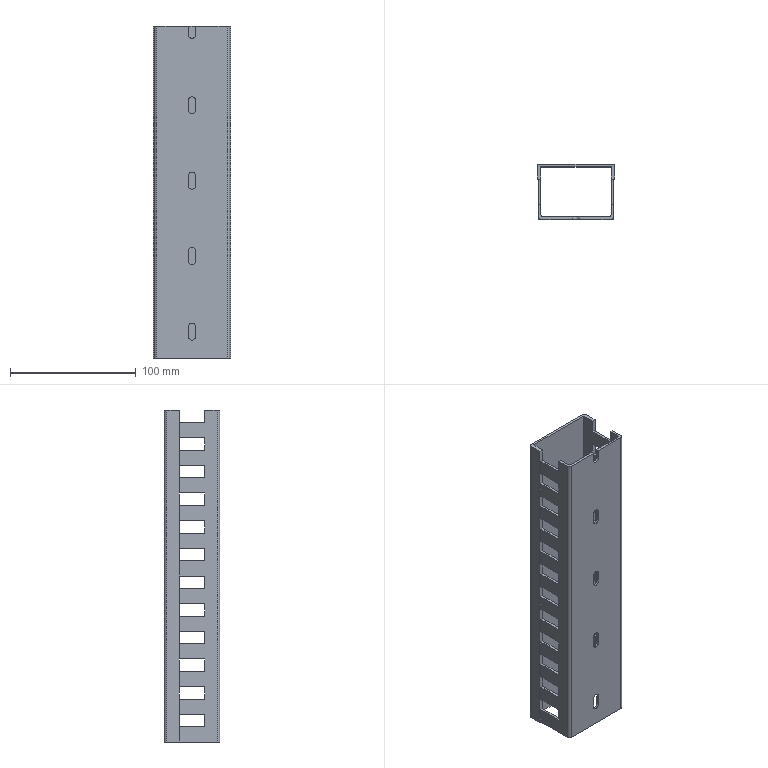Part | STEP file | 11-6060-21411 | 1 solid | 115 faces | box 62 x 44 x 264 mm | volume 101240 mm3 | plane 96 | cylinder 19 | commonest cylinder face diameters 5.5 x13 4 x6